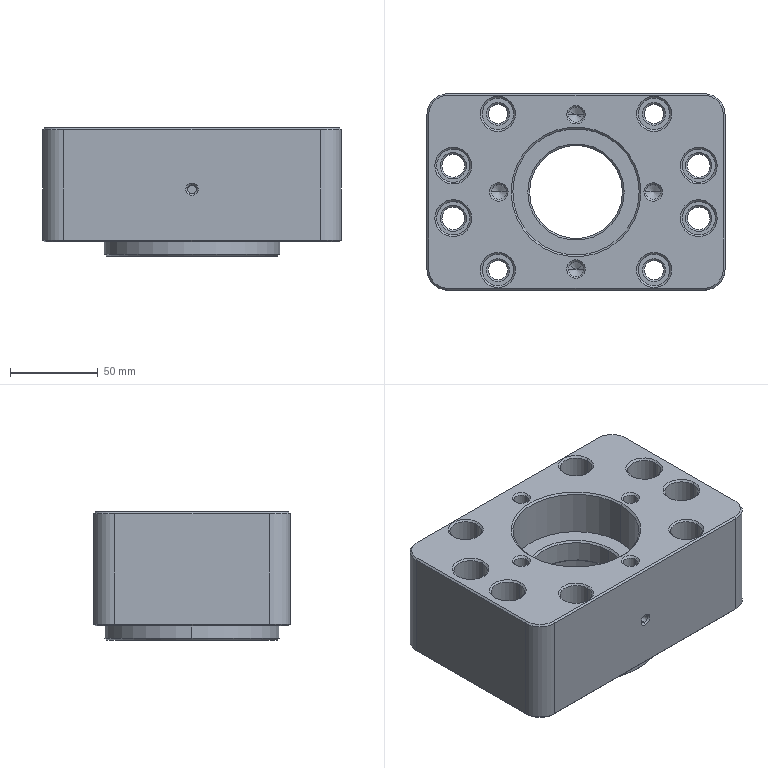NC program | NX | posted with a generic post | part box 170 x 112 x 73 mm
Lines 70 to 734 of 12198:
(HOLE_MILLING , TOOL : D10C)
N120 T10 M6
N122 G54
N124 G17 G0 G90 X-70. Y15. S3500 M3
N126 G43 Z30. H10
N128 Z0.5
N130 G94 G3 X-67.755 Y12.755 R2.245 F1000.
N132 X-65.51 Y15. R2.245
N134 X-65.51 Y15. Z0.3 I-4.49 J0. F2500.
N136 X-65.51 Y15. Z0.1 I-4.49 J0.
N138 X-65.51 Y15. Z-0.1 I-4.49 J0.
N140 X-65.51 Y15. Z-0.3 I-4.49 J0.
N142 X-65.51 Y15. Z-0.5 I-4.49 J0.
N144 X-65.51 Y15. Z-0.7 I-4.49 J0.
N146 X-65.51 Y15. Z-0.9 I-4.49 J0.
N148 X-65.51 Y15. Z-1.1 I-4.49 J0.
N150 X-65.51 Y15. Z-1.3 I-4.49 J0.
N152 X-65.51 Y15. Z-1.5 I-4.49 J0.
N154 X-65.51 Y15. Z-1.7 I-4.49 J0.
N156 X-65.51 Y15. Z-1.9 I-4.49 J0.
N158 X-65.51 Y15. Z-2.1 I-4.49 J0.
N160 X-65.51 Y15. Z-2.3 I-4.49 J0.
N162 X-65.51 Y15. Z-2.5 I-4.49 J0.
N164 X-65.51 Y15. Z-2.7 I-4.49 J0.
N166 X-65.51 Y15. Z-2.9 I-4.49 J0.
N168 X-65.51 Y15. Z-3.1 I-4.49 J0.
N170 X-65.51 Y15. Z-3.3 I-4.49 J0.
N172 X-65.51 Y15. Z-3.5 I-4.49 J0.
N174 X-65.51 Y15. Z-3.7 I-4.49 J0.
N176 X-65.51 Y15. Z-3.9 I-4.49 J0.
N178 X-65.51 Y15. Z-4.1 I-4.49 J0.
N180 X-65.51 Y15. Z-4.3 I-4.49 J0.
N182 X-65.51 Y15. Z-4.5 I-4.49 J0.
N184 X-65.51 Y15. Z-4.7 I-4.49 J0.
N186 X-65.51 Y15. Z-4.9 I-4.49 J0.
N188 X-65.51 Y15. Z-5.1 I-4.49 J0.
N190 X-65.51 Y15. Z-5.3 I-4.49 J0.
N192 X-65.51 Y15. Z-5.5 I-4.49 J0.
N194 X-65.51 Y15. Z-5.7 I-4.49 J0.
N196 X-65.51 Y15. Z-5.9 I-4.49 J0.
N198 X-65.51 Y15. Z-6.1 I-4.49 J0.
N200 X-65.51 Y15. Z-6.3 I-4.49 J0.
N202 X-65.51 Y15. Z-6.5 I-4.49 J0.
N204 X-65.51 Y15. Z-6.7 I-4.49 J0.
N206 X-65.51 Y15. Z-6.9 I-4.49 J0.
N208 X-65.51 Y15. Z-7.1 I-4.49 J0.
N210 X-65.51 Y15. Z-7.3 I-4.49 J0.
N212 X-65.51 Y15. Z-7.5 I-4.49 J0.
N214 X-65.51 Y15. Z-7.7 I-4.49 J0.
N216 X-65.51 Y15. Z-7.9 I-4.49 J0.
N218 X-65.51 Y15. Z-8.1 I-4.49 J0.
N220 X-65.51 Y15. Z-8.3 I-4.49 J0.
N222 X-65.51 Y15. Z-8.5 I-4.49 J0.
N224 X-65.51 Y15. Z-8.7 I-4.49 J0.
N226 X-65.51 Y15. Z-8.9 I-4.49 J0.
N228 X-65.51 Y15. Z-9.1 I-4.49 J0.
N230 X-65.51 Y15. Z-9.3 I-4.49 J0.
N232 X-65.51 Y15. Z-9.5 I-4.49 J0.
N234 X-65.51 Y15. Z-9.7 I-4.49 J0.
N236 X-65.51 Y15. Z-9.9 I-4.49 J0.
N238 X-65.51 Y15. Z-10.1 I-4.49 J0.
N240 X-65.51 Y15. Z-10.3 I-4.49 J0.
N242 X-65.51 Y15. Z-10.5 I-4.49 J0.
N244 X-65.51 Y15. Z-10.7 I-4.49 J0.
N246 X-65.51 Y15. Z-10.9 I-4.49 J0.
N248 X-65.51 Y15. Z-11.1 I-4.49 J0.
N250 X-65.51 Y15. Z-11.3 I-4.49 J0.
N252 X-65.51 Y15. Z-11.5 I-4.49 J0.
N254 X-65.51 Y15. Z-11.7 I-4.49 J0.
N256 X-65.51 Y15. Z-11.9 I-4.49 J0.
N258 X-65.51 Y15. Z-12.1 I-4.49 J0.
N260 X-65.51 Y15. Z-12.3 I-4.49 J0.
N262 X-65.51 Y15. Z-12.5 I-4.49 J0.
N264 X-65.51 Y15. Z-12.7 I-4.49 J0.
N266 X-65.51 Y15. Z-12.9 I-4.49 J0.
N268 X-65.51 Y15. Z-13.1 I-4.49 J0.
N270 X-65.51 Y15. Z-13.3 I-4.49 J0.
N272 X-65.51 Y15. Z-13.5 I-4.49 J0.
N274 X-65.51 Y15. Z-13.7 I-4.49 J0.
N276 X-65.51 Y15. Z-13.9 I-4.49 J0.
N278 X-65.51 Y15. Z-14.1 I-4.49 J0.
N280 X-65.51 Y15. Z-14.3 I-4.49 J0.
N282 X-65.51 Y15. Z-14.5 I-4.49 J0.
N284 X-65.51 Y15. Z-14.7 I-4.49 J0.
N286 X-65.51 Y15. Z-14.9 I-4.49 J0.
N288 X-65.51 Y15. Z-15.1 I-4.49 J0.
N290 X-65.51 Y15. Z-15.3 I-4.49 J0.
N292 X-65.51 Y15. Z-15.5 I-4.49 J0.
N294 X-65.51 Y15. Z-15.7 I-4.49 J0.
N296 X-65.51 Y15. Z-15.9 I-4.49 J0.
N298 X-65.51 Y15. Z-16.1 I-4.49 J0.
N300 X-65.51 Y15. Z-16.3 I-4.49 J0.
N302 X-65.51 Y15. Z-16.5 I-4.49 J0.
N304 X-65.51 Y15. Z-16.7 I-4.49 J0.
N306 X-65.51 Y15. Z-16.9 I-4.49 J0.
N308 X-65.51 Y15. Z-17.1 I-4.49 J0.
N310 X-65.51 Y15. Z-17.3 I-4.49 J0.
N312 X-65.51 Y15. Z-17.5 I-4.49 J0.
N314 X-65.51 Y15. Z-17.7 I-4.49 J0.
N316 X-65.51 Y15. Z-17.9 I-4.49 J0.
N318 X-65.51 Y15. Z-18.1 I-4.49 J0.
N320 X-65.51 Y15. Z-18.3 I-4.49 J0.
N322 X-65.51 Y15. Z-18.5 I-4.49 J0.
N324 X-65.51 Y15. Z-18.7 I-4.49 J0.
N326 X-65.51 Y15. Z-18.9 I-4.49 J0.
N328 X-65.51 Y15. Z-19.1 I-4.49 J0.
N330 X-65.51 Y15. Z-19.3 I-4.49 J0.
N332 X-65.51 Y15. Z-19.5 I-4.49 J0.
N334 X-65.51 Y15. Z-19.7 I-4.49 J0.
N336 X-65.51 Y15. Z-19.9 I-4.49 J0.
N338 X-65.51 Y15. Z-20.1 I-4.49 J0.
N340 X-65.51 Y15. Z-20.3 I-4.49 J0.
N342 X-65.51 Y15. Z-20.5 I-4.49 J0.
N344 X-65.51 Y15. Z-20.7 I-4.49 J0.
N346 X-65.51 Y15. Z-20.9 I-4.49 J0.
N348 X-65.51 Y15. Z-21.1 I-4.49 J0.
N350 X-65.51 Y15. Z-21.3 I-4.49 J0.
N352 X-65.51 Y15. Z-21.5 I-4.49 J0.
N354 X-65.51 Y15. Z-21.7 I-4.49 J0.
N356 X-65.51 Y15. Z-21.9 I-4.49 J0.
N358 X-65.51 Y15. Z-22.1 I-4.49 J0.
N360 X-65.51 Y15. Z-22.3 I-4.49 J0.
N362 X-65.51 Y15. Z-22.5 I-4.49 J0.
N364 X-65.51 Y15. Z-22.7 I-4.49 J0.
N366 X-65.51 Y15. Z-22.9 I-4.49 J0.
N368 X-65.51 Y15. Z-23.1 I-4.49 J0.
N370 X-65.51 Y15. Z-23.3 I-4.49 J0.
N372 X-65.51 Y15. Z-23.5 I-4.49 J0.
N374 X-65.51 Y15. Z-23.7 I-4.49 J0.
N376 X-65.51 Y15. Z-23.9 I-4.49 J0.
N378 X-65.51 Y15. Z-24.1 I-4.49 J0.
N380 X-65.51 Y15. Z-24.3 I-4.49 J0.
N382 X-65.51 Y15. Z-24.5 I-4.49 J0.
N384 X-65.51 Y15. Z-24.7 I-4.49 J0.
N386 X-65.51 Y15. Z-24.9 I-4.49 J0.
N388 X-65.51 Y15. Z-25.1 I-4.49 J0.
N390 X-65.51 Y15. Z-25.3 I-4.49 J0.
N392 X-65.51 Y15. Z-25.5 I-4.49 J0.
N394 X-65.51 Y15. Z-25.7 I-4.49 J0.
N396 X-65.51 Y15. Z-25.9 I-4.49 J0.
N398 X-65.51 Y15. Z-26.1 I-4.49 J0.
N400 X-65.51 Y15. Z-26.3 I-4.49 J0.
N402 X-65.51 Y15. Z-26.5 I-4.49 J0.
N404 X-65.51 Y15. Z-26.7 I-4.49 J0.
N406 X-65.51 Y15. Z-26.9 I-4.49 J0.
N408 X-65.51 Y15. Z-27.1 I-4.49 J0.
N410 X-65.51 Y15. Z-27.3 I-4.49 J0.
N412 X-65.51 Y15. Z-27.5 I-4.49 J0.
N414 X-65.51 Y15. Z-27.7 I-4.49 J0.
N416 X-65.51 Y15. Z-27.9 I-4.49 J0.
N418 X-65.51 Y15. Z-28.1 I-4.49 J0.
N420 X-65.51 Y15. Z-28.3 I-4.49 J0.
N422 X-65.51 Y15. Z-28.5 I-4.49 J0.
N424 X-65.51 Y15. Z-28.7 I-4.49 J0.
N426 X-65.51 Y15. Z-28.9 I-4.49 J0.
N428 X-65.51 Y15. Z-29.1 I-4.49 J0.
N430 X-65.51 Y15. Z-29.3 I-4.49 J0.
N432 X-65.51 Y15. Z-29.5 I-4.49 J0.
N434 X-65.51 Y15. Z-29.7 I-4.49 J0.
N436 X-65.51 Y15. Z-29.9 I-4.49 J0.
N438 X-65.51 Y15. Z-30.1 I-4.49 J0.
N440 X-65.51 Y15. Z-30.3 I-4.49 J0.
N442 X-65.51 Y15. Z-30.5 I-4.49 J0.
N444 X-65.51 Y15. Z-30.7 I-4.49 J0.
N446 X-65.51 Y15. Z-30.9 I-4.49 J0.
N448 X-65.51 Y15. Z-31.1 I-4.49 J0.
N450 X-65.51 Y15. Z-31.3 I-4.49 J0.
N452 X-65.51 Y15. Z-31.5 I-4.49 J0.
N454 X-65.51 Y15. Z-31.7 I-4.49 J0.
N456 X-65.51 Y15. Z-31.9 I-4.49 J0.
N458 X-65.51 Y15. Z-32.1 I-4.49 J0.
N460 X-65.51 Y15. Z-32.3 I-4.49 J0.
N462 X-65.51 Y15. Z-32.5 I-4.49 J0.
N464 X-65.51 Y15. Z-32.7 I-4.49 J0.
N466 X-65.51 Y15. Z-32.9 I-4.49 J0.
N468 X-65.51 Y15. Z-33.1 I-4.49 J0.
N470 X-65.51 Y15. Z-33.3 I-4.49 J0.
N472 X-65.51 Y15. Z-33.5 I-4.49 J0.
N474 X-65.51 Y15. Z-33.7 I-4.49 J0.
N476 X-65.51 Y15. Z-33.9 I-4.49 J0.
N478 X-65.51 Y15. Z-34.1 I-4.49 J0.
N480 X-65.51 Y15. Z-34.3 I-4.49 J0.
N482 X-65.51 Y15. Z-34.5 I-4.49 J0.
N484 X-65.51 Y15. Z-34.7 I-4.49 J0.
N486 X-65.51 Y15. Z-34.9 I-4.49 J0.
N488 X-74.49 Y15. Z-35. I-4.49 J0.
N490 X-70. Y10.51 R4.49
N492 X-74.49 Y15. R-4.49
N494 X-72.245 Y12.755 R2.245
N496 X-70. Y15. R2.245
N498 G0 Z30.
N500 X-44.5 Y44.5
N502 Z0.5
N504 G3 X-42.505 Y42.505 R1.995 F1000.
N506 X-40.51 Y44.5 R1.995
N508 X-40.51 Y44.5 Z0.3 I-3.99 J0. F2500.
N510 X-40.51 Y44.5 Z0.1 I-3.99 J0.
N512 X-40.51 Y44.5 Z-0.1 I-3.99 J0.
N514 X-40.51 Y44.5 Z-0.3 I-3.99 J0.
N516 X-40.51 Y44.5 Z-0.5 I-3.99 J0.
N518 X-40.51 Y44.5 Z-0.7 I-3.99 J0.
N520 X-40.51 Y44.5 Z-0.9 I-3.99 J0.
N522 X-40.51 Y44.5 Z-1.1 I-3.99 J0.
N524 X-40.51 Y44.5 Z-1.3 I-3.99 J0.
N526 X-40.51 Y44.5 Z-1.5 I-3.99 J0.
N528 X-40.51 Y44.5 Z-1.7 I-3.99 J0.
N530 X-40.51 Y44.5 Z-1.9 I-3.99 J0.
N532 X-40.51 Y44.5 Z-2.1 I-3.99 J0.
N534 X-40.51 Y44.5 Z-2.3 I-3.99 J0.
N536 X-40.51 Y44.5 Z-2.5 I-3.99 J0.
N538 X-40.51 Y44.5 Z-2.7 I-3.99 J0.
N540 X-40.51 Y44.5 Z-2.9 I-3.99 J0.
N542 X-40.51 Y44.5 Z-3.1 I-3.99 J0.
N544 X-40.51 Y44.5 Z-3.3 I-3.99 J0.
N546 X-40.51 Y44.5 Z-3.5 I-3.99 J0.
N548 X-40.51 Y44.5 Z-3.7 I-3.99 J0.
N550 X-40.51 Y44.5 Z-3.9 I-3.99 J0.
N552 X-40.51 Y44.5 Z-4.1 I-3.99 J0.
N554 X-40.51 Y44.5 Z-4.3 I-3.99 J0.
N556 X-40.51 Y44.5 Z-4.5 I-3.99 J0.
N558 X-40.51 Y44.5 Z-4.7 I-3.99 J0.
N560 X-40.51 Y44.5 Z-4.9 I-3.99 J0.
N562 X-40.51 Y44.5 Z-5.1 I-3.99 J0.
N564 X-40.51 Y44.5 Z-5.3 I-3.99 J0.
N566 X-40.51 Y44.5 Z-5.5 I-3.99 J0.
N568 X-40.51 Y44.5 Z-5.7 I-3.99 J0.
N570 X-40.51 Y44.5 Z-5.9 I-3.99 J0.
N572 X-40.51 Y44.5 Z-6.1 I-3.99 J0.
N574 X-40.51 Y44.5 Z-6.3 I-3.99 J0.
N576 X-40.51 Y44.5 Z-6.5 I-3.99 J0.
N578 X-40.51 Y44.5 Z-6.7 I-3.99 J0.
N580 X-40.51 Y44.5 Z-6.9 I-3.99 J0.
N582 X-40.51 Y44.5 Z-7.1 I-3.99 J0.
N584 X-40.51 Y44.5 Z-7.3 I-3.99 J0.
N586 X-40.51 Y44.5 Z-7.5 I-3.99 J0.
N588 X-40.51 Y44.5 Z-7.7 I-3.99 J0.
N590 X-40.51 Y44.5 Z-7.9 I-3.99 J0.
N592 X-40.51 Y44.5 Z-8.1 I-3.99 J0.
N594 X-40.51 Y44.5 Z-8.3 I-3.99 J0.
N596 X-40.51 Y44.5 Z-8.5 I-3.99 J0.
N598 X-40.51 Y44.5 Z-8.7 I-3.99 J0.
N600 X-40.51 Y44.5 Z-8.9 I-3.99 J0.
N602 X-40.51 Y44.5 Z-9.1 I-3.99 J0.
N604 X-40.51 Y44.5 Z-9.3 I-3.99 J0.
N606 X-40.51 Y44.5 Z-9.5 I-3.99 J0.
N608 X-40.51 Y44.5 Z-9.7 I-3.99 J0.
N610 X-40.51 Y44.5 Z-9.9 I-3.99 J0.
N612 X-40.51 Y44.5 Z-10.1 I-3.99 J0.
N614 X-40.51 Y44.5 Z-10.3 I-3.99 J0.
N616 X-40.51 Y44.5 Z-10.5 I-3.99 J0.
N618 X-40.51 Y44.5 Z-10.7 I-3.99 J0.
N620 X-40.51 Y44.5 Z-10.9 I-3.99 J0.
N622 X-40.51 Y44.5 Z-11.1 I-3.99 J0.
N624 X-40.51 Y44.5 Z-11.3 I-3.99 J0.
N626 X-40.51 Y44.5 Z-11.5 I-3.99 J0.
N628 X-40.51 Y44.5 Z-11.7 I-3.99 J0.
N630 X-40.51 Y44.5 Z-11.9 I-3.99 J0.
N632 X-40.51 Y44.5 Z-12.1 I-3.99 J0.
N634 X-40.51 Y44.5 Z-12.3 I-3.99 J0.
N636 X-40.51 Y44.5 Z-12.5 I-3.99 J0.
N638 X-40.51 Y44.5 Z-12.7 I-3.99 J0.
N640 X-40.51 Y44.5 Z-12.9 I-3.99 J0.
N642 X-40.51 Y44.5 Z-13.1 I-3.99 J0.
N644 X-40.51 Y44.5 Z-13.3 I-3.99 J0.
N646 X-40.51 Y44.5 Z-13.5 I-3.99 J0.
N648 X-40.51 Y44.5 Z-13.7 I-3.99 J0.
N650 X-40.51 Y44.5 Z-13.9 I-3.99 J0.
N652 X-40.51 Y44.5 Z-14.1 I-3.99 J0.
N654 X-40.51 Y44.5 Z-14.3 I-3.99 J0.
N656 X-40.51 Y44.5 Z-14.5 I-3.99 J0.
N658 X-40.51 Y44.5 Z-14.7 I-3.99 J0.
N660 X-40.51 Y44.5 Z-14.9 I-3.99 J0.
N662 X-40.51 Y44.5 Z-15.1 I-3.99 J0.
N664 X-40.51 Y44.5 Z-15.3 I-3.99 J0.
N666 X-40.51 Y44.5 Z-15.5 I-3.99 J0.
N668 X-40.51 Y44.5 Z-15.7 I-3.99 J0.
N670 X-40.51 Y44.5 Z-15.9 I-3.99 J0.
N672 X-40.51 Y44.5 Z-16.1 I-3.99 J0.
N674 X-40.51 Y44.5 Z-16.3 I-3.99 J0.
N676 X-40.51 Y44.5 Z-16.5 I-3.99 J0.
N678 X-40.51 Y44.5 Z-16.7 I-3.99 J0.
N680 X-40.51 Y44.5 Z-16.9 I-3.99 J0.
N682 X-40.51 Y44.5 Z-17.1 I-3.99 J0.
N684 X-40.51 Y44.5 Z-17.3 I-3.99 J0.
N686 X-40.51 Y44.5 Z-17.5 I-3.99 J0.
N688 X-40.51 Y44.5 Z-17.7 I-3.99 J0.
N690 X-40.51 Y44.5 Z-17.9 I-3.99 J0.
N692 X-40.51 Y44.5 Z-18.1 I-3.99 J0.
N694 X-40.51 Y44.5 Z-18.3 I-3.99 J0.
N696 X-40.51 Y44.5 Z-18.5 I-3.99 J0.
N698 X-40.51 Y44.5 Z-18.7 I-3.99 J0.
N700 X-40.51 Y44.5 Z-18.9 I-3.99 J0.
N702 X-40.51 Y44.5 Z-19.1 I-3.99 J0.
N704 X-40.51 Y44.5 Z-19.3 I-3.99 J0.
N706 X-40.51 Y44.5 Z-19.5 I-3.99 J0.
N708 X-40.51 Y44.5 Z-19.7 I-3.99 J0.
N710 X-40.51 Y44.5 Z-19.9 I-3.99 J0.
N712 X-40.51 Y44.5 Z-20.1 I-3.99 J0.
N714 X-40.51 Y44.5 Z-20.3 I-3.99 J0.
N716 X-40.51 Y44.5 Z-20.5 I-3.99 J0.
N718 X-40.51 Y44.5 Z-20.7 I-3.99 J0.
N720 X-40.51 Y44.5 Z-20.9 I-3.99 J0.
N722 X-40.51 Y44.5 Z-21.1 I-3.99 J0.
N724 X-40.51 Y44.5 Z-21.3 I-3.99 J0.
N726 X-40.51 Y44.5 Z-21.5 I-3.99 J0.
N728 X-40.51 Y44.5 Z-21.7 I-3.99 J0.
N730 X-40.51 Y44.5 Z-21.9 I-3.99 J0.
N732 X-40.51 Y44.5 Z-22.1 I-3.99 J0.
N734 X-40.51 Y44.5 Z-22.3 I-3.99 J0.
N736 X-40.51 Y44.5 Z-22.5 I-3.99 J0.
N738 X-40.51 Y44.5 Z-22.7 I-3.99 J0.
N740 X-40.51 Y44.5 Z-22.9 I-3.99 J0.
N742 X-40.51 Y44.5 Z-23.1 I-3.99 J0.
N744 X-40.51 Y44.5 Z-23.3 I-3.99 J0.
N746 X-40.51 Y44.5 Z-23.5 I-3.99 J0.
N748 X-40.51 Y44.5 Z-23.7 I-3.99 J0.
N750 X-40.51 Y44.5 Z-23.9 I-3.99 J0.
N752 X-40.51 Y44.5 Z-24.1 I-3.99 J0.
N754 X-40.51 Y44.5 Z-24.3 I-3.99 J0.
N756 X-40.51 Y44.5 Z-24.5 I-3.99 J0.
N758 X-40.51 Y44.5 Z-24.7 I-3.99 J0.
N760 X-40.51 Y44.5 Z-24.9 I-3.99 J0.
N762 X-40.51 Y44.5 Z-25.1 I-3.99 J0.
N764 X-40.51 Y44.5 Z-25.3 I-3.99 J0.
N766 X-40.51 Y44.5 Z-25.5 I-3.99 J0.
N768 X-40.51 Y44.5 Z-25.7 I-3.99 J0.
N770 X-40.51 Y44.5 Z-25.9 I-3.99 J0.
N772 X-40.51 Y44.5 Z-26.1 I-3.99 J0.
N774 X-40.51 Y44.5 Z-26.3 I-3.99 J0.
N776 X-40.51 Y44.5 Z-26.5 I-3.99 J0.
N778 X-40.51 Y44.5 Z-26.7 I-3.99 J0.
N780 X-40.51 Y44.5 Z-26.9 I-3.99 J0.
N782 X-40.51 Y44.5 Z-27.1 I-3.99 J0.
N784 X-40.51 Y44.5 Z-27.3 I-3.99 J0.
N786 X-40.51 Y44.5 Z-27.5 I-3.99 J0.
N788 X-40.51 Y44.5 Z-27.7 I-3.99 J0.
N790 X-40.51 Y44.5 Z-27.9 I-3.99 J0.
N792 X-40.51 Y44.5 Z-28.1 I-3.99 J0.
N794 X-40.51 Y44.5 Z-28.3 I-3.99 J0.
N796 X-40.51 Y44.5 Z-28.5 I-3.99 J0.
N798 X-40.51 Y44.5 Z-28.7 I-3.99 J0.
N800 X-40.51 Y44.5 Z-28.9 I-3.99 J0.
N802 X-40.51 Y44.5 Z-29.1 I-3.99 J0.
N804 X-40.51 Y44.5 Z-29.3 I-3.99 J0.
N806 X-40.51 Y44.5 Z-29.5 I-3.99 J0.
N808 X-40.51 Y44.5 Z-29.7 I-3.99 J0.
N810 X-40.51 Y44.5 Z-29.9 I-3.99 J0.
N812 X-40.51 Y44.5 Z-30.1 I-3.99 J0.
N814 X-40.51 Y44.5 Z-30.3 I-3.99 J0.
N816 X-40.51 Y44.5 Z-30.5 I-3.99 J0.
N818 X-40.51 Y44.5 Z-30.7 I-3.99 J0.
N820 X-40.51 Y44.5 Z-30.9 I-3.99 J0.
N822 X-40.51 Y44.5 Z-31.1 I-3.99 J0.
N824 X-40.51 Y44.5 Z-31.3 I-3.99 J0.
N826 X-40.51 Y44.5 Z-31.5 I-3.99 J0.
N828 X-40.51 Y44.5 Z-31.7 I-3.99 J0.
N830 X-40.51 Y44.5 Z-31.9 I-3.99 J0.
N832 X-40.51 Y44.5 Z-32.1 I-3.99 J0.
N834 X-40.51 Y44.5 Z-32.3 I-3.99 J0.
N836 X-40.51 Y44.5 Z-32.5 I-3.99 J0.
N838 X-40.51 Y44.5 Z-32.7 I-3.99 J0.
N840 X-40.51 Y44.5 Z-32.9 I-3.99 J0.
N842 X-40.51 Y44.5 Z-33.1 I-3.99 J0.
N844 X-40.51 Y44.5 Z-33.3 I-3.99 J0.
N846 X-40.51 Y44.5 Z-33.5 I-3.99 J0.
N848 X-40.51 Y44.5 Z-33.7 I-3.99 J0.
N850 X-40.51 Y44.5 Z-33.9 I-3.99 J0.
N852 X-40.51 Y44.5 Z-34.1 I-3.99 J0.
N854 X-40.51 Y44.5 Z-34.3 I-3.99 J0.
N856 X-40.51 Y44.5 Z-34.5 I-3.99 J0.
N858 X-40.51 Y44.5 Z-34.7 I-3.99 J0.
N860 X-40.51 Y44.5 Z-34.9 I-3.99 J0.
N862 X-48.49 Y44.5 Z-35. I-3.99 J0.
N864 X-44.5 Y40.51 R3.99
N866 X-48.49 Y44.5 R-3.99
N868 X-46.495 Y42.505 R1.995
N870 X-44.5 Y44.5 R1.995
N872 G0 Z30.
N874 X-70. Y-15.
N876 Z0.5
N878 G3 X-67.755 Y-17.245 R2.245 F1000.
N880 X-65.51 Y-15. R2.245
N882 X-65.51 Y-15. Z0.3 I-4.49 J0. F2500.
N884 X-65.51 Y-15. Z0.1 I-4.49 J0.
N886 X-65.51 Y-15. Z-0.1 I-4.49 J0.
N888 X-65.51 Y-15. Z-0.3 I-4.49 J0.
N890 X-65.51 Y-15. Z-0.5 I-4.49 J0.
N892 X-65.51 Y-15. Z-0.7 I-4.49 J0.
N894 X-65.51 Y-15. Z-0.9 I-4.49 J0.
N896 X-65.51 Y-15. Z-1.1 I-4.49 J0.
N898 X-65.51 Y-15. Z-1.3 I-4.49 J0.
N900 X-65.51 Y-15. Z-1.5 I-4.49 J0.
N902 X-65.51 Y-15. Z-1.7 I-4.49 J0.
N904 X-65.51 Y-15. Z-1.9 I-4.49 J0.
N906 X-65.51 Y-15. Z-2.1 I-4.49 J0.
N908 X-65.51 Y-15. Z-2.3 I-4.49 J0.
N910 X-65.51 Y-15. Z-2.5 I-4.49 J0.
N912 X-65.51 Y-15. Z-2.7 I-4.49 J0.
N914 X-65.51 Y-15. Z-2.9 I-4.49 J0.
N916 X-65.51 Y-15. Z-3.1 I-4.49 J0.
N918 X-65.51 Y-15. Z-3.3 I-4.49 J0.
N920 X-65.51 Y-15. Z-3.5 I-4.49 J0.
N922 X-65.51 Y-15. Z-3.7 I-4.49 J0.
N924 X-65.51 Y-15. Z-3.9 I-4.49 J0.
N926 X-65.51 Y-15. Z-4.1 I-4.49 J0.
N928 X-65.51 Y-15. Z-4.3 I-4.49 J0.
N930 X-65.51 Y-15. Z-4.5 I-4.49 J0.
N932 X-65.51 Y-15. Z-4.7 I-4.49 J0.
N934 X-65.51 Y-15. Z-4.9 I-4.49 J0.
N936 X-65.51 Y-15. Z-5.1 I-4.49 J0.
N938 X-65.51 Y-15. Z-5.3 I-4.49 J0.
N940 X-65.51 Y-15. Z-5.5 I-4.49 J0.
N942 X-65.51 Y-15. Z-5.7 I-4.49 J0.
N944 X-65.51 Y-15. Z-5.9 I-4.49 J0.
N946 X-65.51 Y-15. Z-6.1 I-4.49 J0.
N948 X-65.51 Y-15. Z-6.3 I-4.49 J0.
N950 X-65.51 Y-15. Z-6.5 I-4.49 J0.
N952 X-65.51 Y-15. Z-6.7 I-4.49 J0.
N954 X-65.51 Y-15. Z-6.9 I-4.49 J0.
N956 X-65.51 Y-15. Z-7.1 I-4.49 J0.
N958 X-65.51 Y-15. Z-7.3 I-4.49 J0.
N960 X-65.51 Y-15. Z-7.5 I-4.49 J0.
N962 X-65.51 Y-15. Z-7.7 I-4.49 J0.
N964 X-65.51 Y-15. Z-7.9 I-4.49 J0.
N966 X-65.51 Y-15. Z-8.1 I-4.49 J0.
N968 X-65.51 Y-15. Z-8.3 I-4.49 J0.
N970 X-65.51 Y-15. Z-8.5 I-4.49 J0.
N972 X-65.51 Y-15. Z-8.7 I-4.49 J0.
N974 X-65.51 Y-15. Z-8.9 I-4.49 J0.
N976 X-65.51 Y-15. Z-9.1 I-4.49 J0.
N978 X-65.51 Y-15. Z-9.3 I-4.49 J0.
N980 X-65.51 Y-15. Z-9.5 I-4.49 J0.
N982 X-65.51 Y-15. Z-9.7 I-4.49 J0.
N984 X-65.51 Y-15. Z-9.9 I-4.49 J0.
N986 X-65.51 Y-15. Z-10.1 I-4.49 J0.
N988 X-65.51 Y-15. Z-10.3 I-4.49 J0.
N990 X-65.51 Y-15. Z-10.5 I-4.49 J0.
N992 X-65.51 Y-15. Z-10.7 I-4.49 J0.
N994 X-65.51 Y-15. Z-10.9 I-4.49 J0.
N996 X-65.51 Y-15. Z-11.1 I-4.49 J0.
N998 X-65.51 Y-15. Z-11.3 I-4.49 J0.
N1000 X-65.51 Y-15. Z-11.5 I-4.49 J0.
N1002 X-65.51 Y-15. Z-11.7 I-4.49 J0.
N1004 X-65.51 Y-15. Z-11.9 I-4.49 J0.
N1006 X-65.51 Y-15. Z-12.1 I-4.49 J0.
N1008 X-65.51 Y-15. Z-12.3 I-4.49 J0.
N1010 X-65.51 Y-15. Z-12.5 I-4.49 J0.
N1012 X-65.51 Y-15. Z-12.7 I-4.49 J0.
N1014 X-65.51 Y-15. Z-12.9 I-4.49 J0.
N1016 X-65.51 Y-15. Z-13.1 I-4.49 J0.
N1018 X-65.51 Y-15. Z-13.3 I-4.49 J0.
N1020 X-65.51 Y-15. Z-13.5 I-4.49 J0.
N1022 X-65.51 Y-15. Z-13.7 I-4.49 J0.
N1024 X-65.51 Y-15. Z-13.9 I-4.49 J0.
N1026 X-65.51 Y-15. Z-14.1 I-4.49 J0.
N1028 X-65.51 Y-15. Z-14.3 I-4.49 J0.
N1030 X-65.51 Y-15. Z-14.5 I-4.49 J0.
N1032 X-65.51 Y-15. Z-14.7 I-4.49 J0.
N1034 X-65.51 Y-15. Z-14.9 I-4.49 J0.
N1036 X-65.51 Y-15. Z-15.1 I-4.49 J0.
N1038 X-65.51 Y-15. Z-15.3 I-4.49 J0.
N1040 X-65.51 Y-15. Z-15.5 I-4.49 J0.
N1042 X-65.51 Y-15. Z-15.7 I-4.49 J0.
N1044 X-65.51 Y-15. Z-15.9 I-4.49 J0.
N1046 X-65.51 Y-15. Z-16.1 I-4.49 J0.
N1048 X-65.51 Y-15. Z-16.3 I-4.49 J0.
N1050 X-65.51 Y-15. Z-16.5 I-4.49 J0.
N1052 X-65.51 Y-15. Z-16.7 I-4.49 J0.
N1054 X-65.51 Y-15. Z-16.9 I-4.49 J0.
N1056 X-65.51 Y-15. Z-17.1 I-4.49 J0.
N1058 X-65.51 Y-15. Z-17.3 I-4.49 J0.
N1060 X-65.51 Y-15. Z-17.5 I-4.49 J0.
N1062 X-65.51 Y-15. Z-17.7 I-4.49 J0.
N1064 X-65.51 Y-15. Z-17.9 I-4.49 J0.
N1066 X-65.51 Y-15. Z-18.1 I-4.49 J0.
N1068 X-65.51 Y-15. Z-18.3 I-4.49 J0.
N1070 X-65.51 Y-15. Z-18.5 I-4.49 J0.
N1072 X-65.51 Y-15. Z-18.7 I-4.49 J0.
N1074 X-65.51 Y-15. Z-18.9 I-4.49 J0.
N1076 X-65.51 Y-15. Z-19.1 I-4.49 J0.
N1078 X-65.51 Y-15. Z-19.3 I-4.49 J0.
N1080 X-65.51 Y-15. Z-19.5 I-4.49 J0.
N1082 X-65.51 Y-15. Z-19.7 I-4.49 J0.
N1084 X-65.51 Y-15. Z-19.9 I-4.49 J0.
N1086 X-65.51 Y-15. Z-20.1 I-4.49 J0.
N1088 X-65.51 Y-15. Z-20.3 I-4.49 J0.
N1090 X-65.51 Y-15. Z-20.5 I-4.49 J0.
N1092 X-65.51 Y-15. Z-20.7 I-4.49 J0.
N1094 X-65.51 Y-15. Z-20.9 I-4.49 J0.
N1096 X-65.51 Y-15. Z-21.1 I-4.49 J0.
N1098 X-65.51 Y-15. Z-21.3 I-4.49 J0.
N1100 X-65.51 Y-15. Z-21.5 I-4.49 J0.
N1102 X-65.51 Y-15. Z-21.7 I-4.49 J0.
N1104 X-65.51 Y-15. Z-21.9 I-4.49 J0.
N1106 X-65.51 Y-15. Z-22.1 I-4.49 J0.
N1108 X-65.51 Y-15. Z-22.3 I-4.49 J0.
N1110 X-65.51 Y-15. Z-22.5 I-4.49 J0.
N1112 X-65.51 Y-15. Z-22.7 I-4.49 J0.
N1114 X-65.51 Y-15. Z-22.9 I-4.49 J0.
N1116 X-65.51 Y-15. Z-23.1 I-4.49 J0.
N1118 X-65.51 Y-15. Z-23.3 I-4.49 J0.
N1120 X-65.51 Y-15. Z-23.5 I-4.49 J0.
N1122 X-65.51 Y-15. Z-23.7 I-4.49 J0.
N1124 X-65.51 Y-15. Z-23.9 I-4.49 J0.
N1126 X-65.51 Y-15. Z-24.1 I-4.49 J0.
N1128 X-65.51 Y-15. Z-24.3 I-4.49 J0.
N1130 X-65.51 Y-15. Z-24.5 I-4.49 J0.
N1132 X-65.51 Y-15. Z-24.7 I-4.49 J0.
N1134 X-65.51 Y-15. Z-24.9 I-4.49 J0.
N1136 X-65.51 Y-15. Z-25.1 I-4.49 J0.
N1138 X-65.51 Y-15. Z-25.3 I-4.49 J0.
N1140 X-65.51 Y-15. Z-25.5 I-4.49 J0.
N1142 X-65.51 Y-15. Z-25.7 I-4.49 J0.
N1144 X-65.51 Y-15. Z-25.9 I-4.49 J0.
N1146 X-65.51 Y-15. Z-26.1 I-4.49 J0.
N1148 X-65.51 Y-15. Z-26.3 I-4.49 J0.
N1150 X-65.51 Y-15. Z-26.5 I-4.49 J0.
N1152 X-65.51 Y-15. Z-26.7 I-4.49 J0.
N1154 X-65.51 Y-15. Z-26.9 I-4.49 J0.
N1156 X-65.51 Y-15. Z-27.1 I-4.49 J0.
N1158 X-65.51 Y-15. Z-27.3 I-4.49 J0.
N1160 X-65.51 Y-15. Z-27.5 I-4.49 J0.
N1162 X-65.51 Y-15. Z-27.7 I-4.49 J0.
N1164 X-65.51 Y-15. Z-27.9 I-4.49 J0.
N1166 X-65.51 Y-15. Z-28.1 I-4.49 J0.
N1168 X-65.51 Y-15. Z-28.3 I-4.49 J0.
N1170 X-65.51 Y-15. Z-28.5 I-4.49 J0.
N1172 X-65.51 Y-15. Z-28.7 I-4.49 J0.
N1174 X-65.51 Y-15. Z-28.9 I-4.49 J0.
N1176 X-65.51 Y-15. Z-29.1 I-4.49 J0.
N1178 X-65.51 Y-15. Z-29.3 I-4.49 J0.
N1180 X-65.51 Y-15. Z-29.5 I-4.49 J0.
N1182 X-65.51 Y-15. Z-29.7 I-4.49 J0.
N1184 X-65.51 Y-15. Z-29.9 I-4.49 J0.
N1186 X-65.51 Y-15. Z-30.1 I-4.49 J0.
N1188 X-65.51 Y-15. Z-30.3 I-4.49 J0.
N1190 X-65.51 Y-15. Z-30.5 I-4.49 J0.
N1192 X-65.51 Y-15. Z-30.7 I-4.49 J0.
N1194 X-65.51 Y-15. Z-30.9 I-4.49 J0.
N1196 X-65.51 Y-15. Z-31.1 I-4.49 J0.
N1198 X-65.51 Y-15. Z-31.3 I-4.49 J0.
N1200 X-65.51 Y-15. Z-31.5 I-4.49 J0.
N1202 X-65.51 Y-15. Z-31.7 I-4.49 J0.
N1204 X-65.51 Y-15. Z-31.9 I-4.49 J0.
N1206 X-65.51 Y-15. Z-32.1 I-4.49 J0.
N1208 X-65.51 Y-15. Z-32.3 I-4.49 J0.
N1210 X-65.51 Y-15. Z-32.5 I-4.49 J0.
N1212 X-65.51 Y-15. Z-32.7 I-4.49 J0.
N1214 X-65.51 Y-15. Z-32.9 I-4.49 J0.
N1216 X-65.51 Y-15. Z-33.1 I-4.49 J0.
N1218 X-65.51 Y-15. Z-33.3 I-4.49 J0.
N1220 X-65.51 Y-15. Z-33.5 I-4.49 J0.
N1222 X-65.51 Y-15. Z-33.7 I-4.49 J0.
N1224 X-65.51 Y-15. Z-33.9 I-4.49 J0.
N1226 X-65.51 Y-15. Z-34.1 I-4.49 J0.
N1228 X-65.51 Y-15. Z-34.3 I-4.49 J0.
N1230 X-65.51 Y-15. Z-34.5 I-4.49 J0.
N1232 X-65.51 Y-15. Z-34.7 I-4.49 J0.
N1234 X-65.51 Y-15. Z-34.9 I-4.49 J0.
N1236 X-74.49 Y-15. Z-35. I-4.49 J0.
N1238 X-70. Y-19.49 R4.49
N1240 X-74.49 Y-15. R-4.49
N1242 X-72.245 Y-17.245 R2.245
N1244 X-70. Y-15. R2.245
N1246 G0 Z30.
N1248 X-44.5 Y-44.5
N1250 Z0.5
N1252 G3 X-42.505 Y-46.495 R1.995 F1000.
N1254 X-40.51 Y-44.5 R1.995
N1256 X-40.51 Y-44.5 Z0.3 I-3.99 J0. F2500.
N1258 X-40.51 Y-44.5 Z0.1 I-3.99 J0.
N1260 X-40.51 Y-44.5 Z-0.1 I-3.99 J0.
N1262 X-40.51 Y-44.5 Z-0.3 I-3.99 J0.
N1264 X-40.51 Y-44.5 Z-0.5 I-3.99 J0.
N1266 X-40.51 Y-44.5 Z-0.7 I-3.99 J0.
N1268 X-40.51 Y-44.5 Z-0.9 I-3.99 J0.
N1270 X-40.51 Y-44.5 Z-1.1 I-3.99 J0.
N1272 X-40.51 Y-44.5 Z-1.3 I-3.99 J0.
N1274 X-40.51 Y-44.5 Z-1.5 I-3.99 J0.
N1276 X-40.51 Y-44.5 Z-1.7 I-3.99 J0.
N1278 X-40.51 Y-44.5 Z-1.9 I-3.99 J0.
N1280 X-40.51 Y-44.5 Z-2.1 I-3.99 J0.
N1282 X-40.51 Y-44.5 Z-2.3 I-3.99 J0.
N1284 X-40.51 Y-44.5 Z-2.5 I-3.99 J0.
N1286 X-40.51 Y-44.5 Z-2.7 I-3.99 J0.
N1288 X-40.51 Y-44.5 Z-2.9 I-3.99 J0.
N1290 X-40.51 Y-44.5 Z-3.1 I-3.99 J0.
N1292 X-40.51 Y-44.5 Z-3.3 I-3.99 J0.
N1294 X-40.51 Y-44.5 Z-3.5 I-3.99 J0.
N1296 X-40.51 Y-44.5 Z-3.7 I-3.99 J0.
N1298 X-40.51 Y-44.5 Z-3.9 I-3.99 J0.
N1300 X-40.51 Y-44.5 Z-4.1 I-3.99 J0.
N1302 X-40.51 Y-44.5 Z-4.3 I-3.99 J0.
N1304 X-40.51 Y-44.5 Z-4.5 I-3.99 J0.
N1306 X-40.51 Y-44.5 Z-4.7 I-3.99 J0.
N1308 X-40.51 Y-44.5 Z-4.9 I-3.99 J0.
N1310 X-40.51 Y-44.5 Z-5.1 I-3.99 J0.
N1312 X-40.51 Y-44.5 Z-5.3 I-3.99 J0.
N1314 X-40.51 Y-44.5 Z-5.5 I-3.99 J0.
N1316 X-40.51 Y-44.5 Z-5.7 I-3.99 J0.
N1318 X-40.51 Y-44.5 Z-5.9 I-3.99 J0.
N1320 X-40.51 Y-44.5 Z-6.1 I-3.99 J0.
N1322 X-40.51 Y-44.5 Z-6.3 I-3.99 J0.
N1324 X-40.51 Y-44.5 Z-6.5 I-3.99 J0.
N1326 X-40.51 Y-44.5 Z-6.7 I-3.99 J0.
N1328 X-40.51 Y-44.5 Z-6.9 I-3.99 J0.
N1330 X-40.51 Y-44.5 Z-7.1 I-3.99 J0.
N1332 X-40.51 Y-44.5 Z-7.3 I-3.99 J0.
N1334 X-40.51 Y-44.5 Z-7.5 I-3.99 J0.
N1336 X-40.51 Y-44.5 Z-7.7 I-3.99 J0.
N1338 X-40.51 Y-44.5 Z-7.9 I-3.99 J0.
N1340 X-40.51 Y-44.5 Z-8.1 I-3.99 J0.
N1342 X-40.51 Y-44.5 Z-8.3 I-3.99 J0.
N1344 X-40.51 Y-44.5 Z-8.5 I-3.99 J0.
N1346 X-40.51 Y-44.5 Z-8.7 I-3.99 J0.
N1348 X-40.51 Y-44.5 Z-8.9 I-3.99 J0.
N1350 X-40.51 Y-44.5 Z-9.1 I-3.99 J0.
N1352 X-40.51 Y-44.5 Z-9.3 I-3.99 J0.
N1354 X-40.51 Y-44.5 Z-9.5 I-3.99 J0.
N1356 X-40.51 Y-44.5 Z-9.7 I-3.99 J0.
N1358 X-40.51 Y-44.5 Z-9.9 I-3.99 J0.
N1360 X-40.51 Y-44.5 Z-10.1 I-3.99 J0.
N1362 X-40.51 Y-44.5 Z-10.3 I-3.99 J0.
N1364 X-40.51 Y-44.5 Z-10.5 I-3.99 J0.
N1366 X-40.51 Y-44.5 Z-10.7 I-3.99 J0.
N1368 X-40.51 Y-44.5 Z-10.9 I-3.99 J0.
N1370 X-40.51 Y-44.5 Z-11.1 I-3.99 J0.
N1372 X-40.51 Y-44.5 Z-11.3 I-3.99 J0.
N1374 X-40.51 Y-44.5 Z-11.5 I-3.99 J0.
N1376 X-40.51 Y-44.5 Z-11.7 I-3.99 J0.
N1378 X-40.51 Y-44.5 Z-11.9 I-3.99 J0.
N1380 X-40.51 Y-44.5 Z-12.1 I-3.99 J0.
N1382 X-40.51 Y-44.5 Z-12.3 I-3.99 J0.
N1384 X-40.51 Y-44.5 Z-12.5 I-3.99 J0.
N1386 X-40.51 Y-44.5 Z-12.7 I-3.99 J0.
N1388 X-40.51 Y-44.5 Z-12.9 I-3.99 J0.
N1390 X-40.51 Y-44.5 Z-13.1 I-3.99 J0.
N1392 X-40.51 Y-44.5 Z-13.3 I-3.99 J0.
N1394 X-40.51 Y-44.5 Z-13.5 I-3.99 J0.
N1396 X-40.51 Y-44.5 Z-13.7 I-3.99 J0.
N1398 X-40.51 Y-44.5 Z-13.9 I-3.99 J0.
N1400 X-40.51 Y-44.5 Z-14.1 I-3.99 J0.
N1402 X-40.51 Y-44.5 Z-14.3 I-3.99 J0.
N1404 X-40.51 Y-44.5 Z-14.5 I-3.99 J0.
N1406 X-40.51 Y-44.5 Z-14.7 I-3.99 J0.
N1408 X-40.51 Y-44.5 Z-14.9 I-3.99 J0.
N1410 X-40.51 Y-44.5 Z-15.1 I-3.99 J0.
N1412 X-40.51 Y-44.5 Z-15.3 I-3.99 J0.
N1414 X-40.51 Y-44.5 Z-15.5 I-3.99 J0.
N1416 X-40.51 Y-44.5 Z-15.7 I-3.99 J0.
N1418 X-40.51 Y-44.5 Z-15.9 I-3.99 J0.
N1420 X-40.51 Y-44.5 Z-16.1 I-3.99 J0.
N1422 X-40.51 Y-44.5 Z-16.3 I-3.99 J0.
N1424 X-40.51 Y-44.5 Z-16.5 I-3.99 J0.
N1426 X-40.51 Y-44.5 Z-16.7 I-3.99 J0.
N1428 X-40.51 Y-44.5 Z-16.9 I-3.99 J0.
N1430 X-40.51 Y-44.5 Z-17.1 I-3.99 J0.
N1432 X-40.51 Y-44.5 Z-17.3 I-3.99 J0.
N1434 X-40.51 Y-44.5 Z-17.5 I-3.99 J0.
N1436 X-40.51 Y-44.5 Z-17.7 I-3.99 J0.
N1438 X-40.51 Y-44.5 Z-17.9 I-3.99 J0.
N1440 X-40.51 Y-44.5 Z-18.1 I-3.99 J0.
N1442 X-40.51 Y-44.5 Z-18.3 I-3.99 J0.